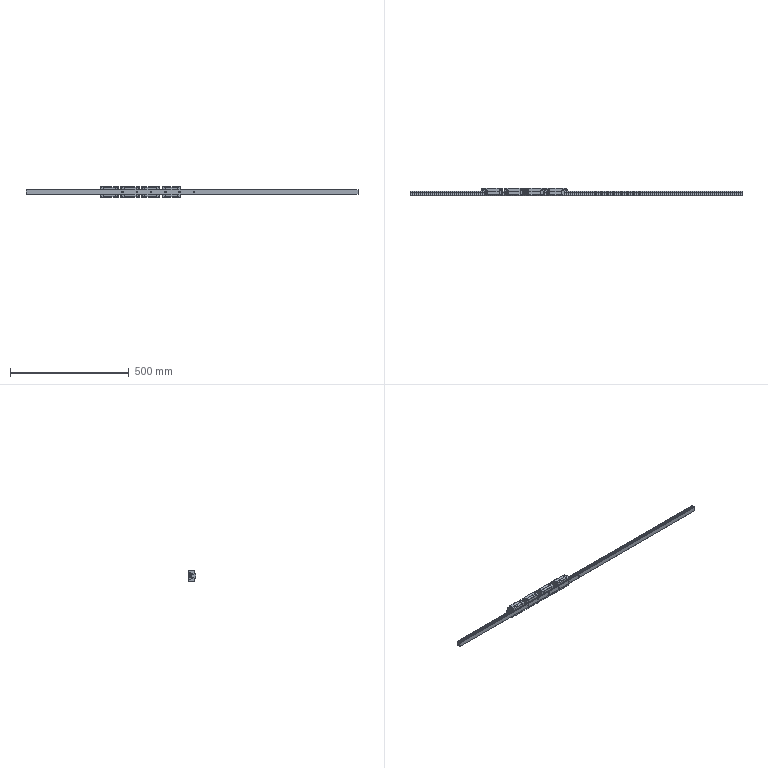Part | SolidWorks | 29 solids | 3223 faces | volume 682203 mm3 | plane 2020 | cylinder 902 | cone 184 | spline 81 | sphere 24 | torus 12 | commonest cylinder face diameters 1 x284 0.2 x136 2 x110 4.06 x84 0.1 x72 6 x60